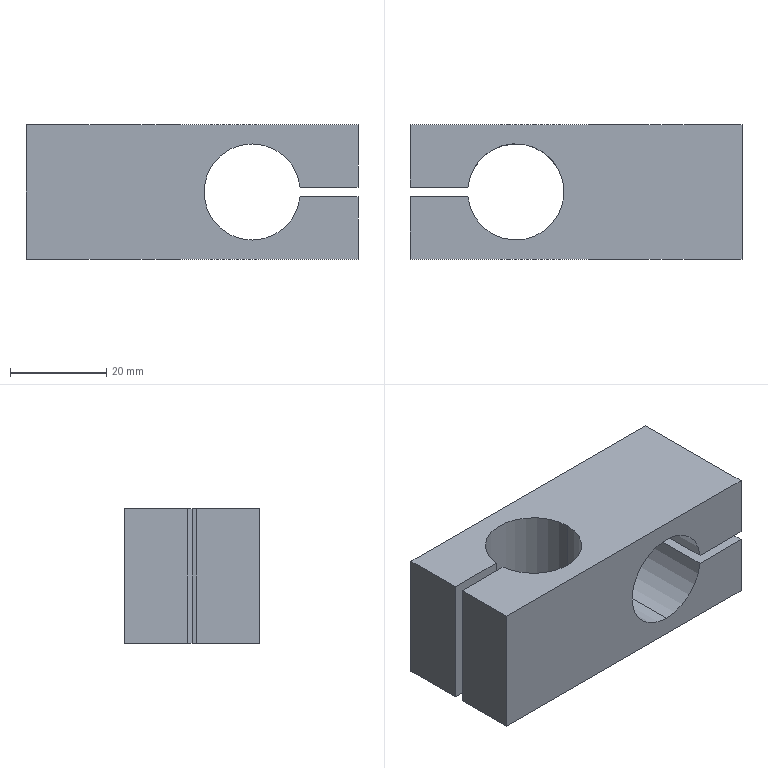Part | SolidWorks | features ICE 2, Extrusion 1 | 1 solid | 17 faces | box 69 x 28 x 28 mm | volume 35157 mm3 | plane 12 | cylinder 5 | commonest cylinder face diameters 20 x5
STEP:
#1=CARTESIAN_POINT('',(12.5,-14.,-10.));
#2=VERTEX_POINT('',#1);
#3=CARTESIAN_POINT('',(12.5,-14.,10.));
#4=VERTEX_POINT('',#3);
#5=CARTESIAN_POINT('',(12.5,-14.,0.));
#6=DIRECTION('',(0.,1.,0.));
#7=DIRECTION('',(0.,0.,1.));
#8=AXIS2_PLACEMENT_3D('',#5,#6,#7);
#9=CIRCLE('',#8,10.);
#10=EDGE_CURVE('',#2,#4,#9,.T.);
#11=ORIENTED_EDGE('',*,*,#10,.F.);
#12=CARTESIAN_POINT('',(12.5,14.,-10.));
#13=VERTEX_POINT('',#12);
#14=CARTESIAN_POINT('',(12.5,-14.,-10.));
#15=DIRECTION('',(0.,1.,0.));
#16=VECTOR('',#15,1000.);
#17=LINE('',#14,#16);
#18=EDGE_CURVE('',#2,#13,#17,.T.);
#19=ORIENTED_EDGE('',*,*,#18,.T.);
#20=CARTESIAN_POINT('',(12.5,14.,10.));
#21=VERTEX_POINT('',#20);
#22=CARTESIAN_POINT('',(12.5,14.,0.));
#23=DIRECTION('',(0.,1.,0.));
#24=DIRECTION('',(0.,0.,1.));
#25=AXIS2_PLACEMENT_3D('',#22,#23,#24);
#26=CIRCLE('',#25,10.);
#27=EDGE_CURVE('',#13,#21,#26,.T.);
#28=ORIENTED_EDGE('',*,*,#27,.T.);
#29=CARTESIAN_POINT('',(12.5,-14.,10.));
#30=DIRECTION('',(0.,1.,0.));
#31=VECTOR('',#30,1000.);
#32=LINE('',#29,#31);
#33=EDGE_CURVE('',#4,#21,#32,.T.);
#34=ORIENTED_EDGE('',*,*,#33,.F.);
#35=EDGE_LOOP('',(#11,#19,#28,#34));
#36=FACE_OUTER_BOUND('',#35,.T.);
#37=CARTESIAN_POINT('',(12.5,-14.,0.));
#38=DIRECTION('',(0.,1.,0.));
#39=DIRECTION('',(0.,0.,1.));
#40=AXIS2_PLACEMENT_3D('',#37,#38,#39);
#41=CYLINDRICAL_SURFACE('',#40,10.);
#42=ADVANCED_FACE('',(#36),#41,.F.);
#43=CARTESIAN_POINT('',(22.45,-14.,1.));
#44=VERTEX_POINT('',#43);
#45=CARTESIAN_POINT('',(12.5,-14.,0.));
#46=DIRECTION('',(0.,1.,0.));
#47=DIRECTION('',(0.,0.,1.));
#48=AXIS2_PLACEMENT_3D('',#45,#46,#47);
#49=CIRCLE('',#48,10.);
#50=EDGE_CURVE('',#4,#44,#49,.T.);
#51=ORIENTED_EDGE('',*,*,#50,.F.);
#52=ORIENTED_EDGE('',*,*,#33,.T.);
#53=CARTESIAN_POINT('',(22.45,14.,1.));
#54=VERTEX_POINT('',#53);
#55=CARTESIAN_POINT('',(12.5,14.,0.));
#56=DIRECTION('',(0.,1.,0.));
#57=DIRECTION('',(0.,0.,1.));
#58=AXIS2_PLACEMENT_3D('',#55,#56,#57);
#59=CIRCLE('',#58,10.);
#60=EDGE_CURVE('',#21,#54,#59,.T.);
#61=ORIENTED_EDGE('',*,*,#60,.T.);
#62=CARTESIAN_POINT('',(22.45,-14.,1.));
#63=DIRECTION('',(0.,1.,0.));
#64=VECTOR('',#63,1000.);
#65=LINE('',#62,#64);
#66=EDGE_CURVE('',#44,#54,#65,.T.);
#67=ORIENTED_EDGE('',*,*,#66,.F.);
#68=EDGE_LOOP('',(#51,#52,#61,#67));
#69=FACE_OUTER_BOUND('',#68,.T.);
#70=CARTESIAN_POINT('',(12.5,-14.,0.));
#71=DIRECTION('',(0.,1.,0.));
#72=DIRECTION('',(0.,0.,1.));
#73=AXIS2_PLACEMENT_3D('',#70,#71,#72);
#74=CYLINDRICAL_SURFACE('',#73,10.);
#75=ADVANCED_FACE('',(#69),#74,.F.);
#76=CARTESIAN_POINT('',(-2.5,0.,-14.));
#77=VERTEX_POINT('',#76);
#78=CARTESIAN_POINT('',(-22.45,1.,-14.));
#79=VERTEX_POINT('',#78);
#80=CARTESIAN_POINT('',(-12.5,0.,-14.));
#81=DIRECTION('',(0.,0.,1.));
#82=DIRECTION('',(1.,0.,0.));
#83=AXIS2_PLACEMENT_3D('',#80,#81,#82);
#84=CIRCLE('',#83,10.);
#85=EDGE_CURVE('',#77,#79,#84,.T.);
#86=ORIENTED_EDGE('',*,*,#85,.F.);
#87=CARTESIAN_POINT('',(-2.5,0.,14.));
#88=VERTEX_POINT('',#87);
#89=CARTESIAN_POINT('',(-2.5,0.,-14.));
#90=DIRECTION('',(0.,0.,1.));
#91=VECTOR('',#90,1000.);
#92=LINE('',#89,#91);
#93=EDGE_CURVE('',#77,#88,#92,.T.);
#94=ORIENTED_EDGE('',*,*,#93,.T.);
#95=CARTESIAN_POINT('',(-22.45,1.,14.));
#96=VERTEX_POINT('',#95);
#97=CARTESIAN_POINT('',(-12.5,0.,14.));
#98=DIRECTION('',(0.,0.,1.));
#99=DIRECTION('',(1.,0.,0.));
#100=AXIS2_PLACEMENT_3D('',#97,#98,#99);
#101=CIRCLE('',#100,10.);
#102=EDGE_CURVE('',#88,#96,#101,.T.);
#103=ORIENTED_EDGE('',*,*,#102,.T.);
#104=CARTESIAN_POINT('',(-22.45,1.,-14.));
#105=DIRECTION('',(0.,0.,1.));
#106=VECTOR('',#105,1000.);
#107=LINE('',#104,#106);
#108=EDGE_CURVE('',#79,#96,#107,.T.);
#109=ORIENTED_EDGE('',*,*,#108,.F.);
#110=EDGE_LOOP('',(#86,#94,#103,#109));
#111=FACE_OUTER_BOUND('',#110,.T.);
#112=CARTESIAN_POINT('',(-12.5,0.,-14.));
#113=DIRECTION('',(0.,0.,1.));
#114=DIRECTION('',(1.,0.,0.));
#115=AXIS2_PLACEMENT_3D('',#112,#113,#114);
#116=CYLINDRICAL_SURFACE('',#115,10.);
#117=ADVANCED_FACE('',(#111),#116,.F.);
#118=CARTESIAN_POINT('',(34.5,14.,-1.));
#119=VERTEX_POINT('',#118);
#120=CARTESIAN_POINT('',(34.5,14.,-14.));
#121=VERTEX_POINT('',#120);
#122=CARTESIAN_POINT('',(34.5,14.,14.));
#123=DIRECTION('',(0.,0.,-1.));
#124=VECTOR('',#123,1000.);
#125=LINE('',#122,#124);
#126=EDGE_CURVE('',#119,#121,#125,.T.);
#127=ORIENTED_EDGE('',*,*,#126,.F.);
#128=CARTESIAN_POINT('',(34.5,-14.,-1.));
#129=VERTEX_POINT('',#128);
#130=CARTESIAN_POINT('',(34.5,-14.,-1.));
#131=DIRECTION('',(0.,1.,0.));
#132=VECTOR('',#131,1000.);
#133=LINE('',#130,#132);
#134=EDGE_CURVE('',#129,#119,#133,.T.);
#135=ORIENTED_EDGE('',*,*,#134,.F.);
#136=CARTESIAN_POINT('',(34.5,-14.,-14.));
#137=VERTEX_POINT('',#136);
#138=CARTESIAN_POINT('',(34.5,-14.,14.));
#139=DIRECTION('',(0.,0.,-1.));
#140=VECTOR('',#139,1000.);
#141=LINE('',#138,#140);
#142=EDGE_CURVE('',#129,#137,#141,.T.);
#143=ORIENTED_EDGE('',*,*,#142,.T.);
#144=CARTESIAN_POINT('',(34.5,14.,-14.));
#145=DIRECTION('',(0.,1.,0.));
#146=VECTOR('',#145,1000.);
#147=LINE('',#144,#146);
#148=EDGE_CURVE('',#137,#121,#147,.T.);
#149=ORIENTED_EDGE('',*,*,#148,.T.);
#150=EDGE_LOOP('',(#127,#135,#143,#149));
#151=FACE_OUTER_BOUND('',#150,.T.);
#152=CARTESIAN_POINT('',(34.5,14.,14.));
#153=DIRECTION('',(-1.,0.,0.));
#154=DIRECTION('',(0.,0.,1.));
#155=AXIS2_PLACEMENT_3D('',#152,#153,#154);
#156=PLANE('',#155);
#157=ADVANCED_FACE('',(#151),#156,.F.);
#158=CARTESIAN_POINT('',(-34.5,14.,-14.));
#159=VERTEX_POINT('',#158);
#160=CARTESIAN_POINT('',(-34.5,1.,-14.));
#161=VERTEX_POINT('',#160);
#162=CARTESIAN_POINT('',(-34.5,14.,-14.));
#163=DIRECTION('',(0.,-1.,0.));
#164=VECTOR('',#163,1000.);
#165=LINE('',#162,#164);
#166=EDGE_CURVE('',#159,#161,#165,.T.);
#167=ORIENTED_EDGE('',*,*,#166,.T.);
#168=CARTESIAN_POINT('',(-34.5,1.,14.));
#169=VERTEX_POINT('',#168);
#170=CARTESIAN_POINT('',(-34.5,1.,-14.));
#171=DIRECTION('',(0.,0.,1.));
#172=VECTOR('',#171,1000.);
#173=LINE('',#170,#172);
#174=EDGE_CURVE('',#161,#169,#173,.T.);
#175=ORIENTED_EDGE('',*,*,#174,.T.);
#176=CARTESIAN_POINT('',(-34.5,14.,14.));
#177=VERTEX_POINT('',#176);
#178=CARTESIAN_POINT('',(-34.5,14.,14.));
#179=DIRECTION('',(0.,-1.,0.));
#180=VECTOR('',#179,1000.);
#181=LINE('',#178,#180);
#182=EDGE_CURVE('',#177,#169,#181,.T.);
#183=ORIENTED_EDGE('',*,*,#182,.F.);
#184=CARTESIAN_POINT('',(-34.5,14.,14.));
#185=DIRECTION('',(0.,0.,-1.));
#186=VECTOR('',#185,1000.);
#187=LINE('',#184,#186);
#188=EDGE_CURVE('',#177,#159,#187,.T.);
#189=ORIENTED_EDGE('',*,*,#188,.T.);
#190=EDGE_LOOP('',(#167,#175,#183,#189));
#191=FACE_OUTER_BOUND('',#190,.T.);
#192=CARTESIAN_POINT('',(-34.5,14.,14.));
#193=DIRECTION('',(1.,0.,0.));
#194=DIRECTION('',(0.,0.,-1.));
#195=AXIS2_PLACEMENT_3D('',#192,#193,#194);
#196=PLANE('',#195);
#197=ADVANCED_FACE('',(#191),#196,.F.);
#198=CARTESIAN_POINT('',(34.5,-14.,14.));
#199=VERTEX_POINT('',#198);
#200=CARTESIAN_POINT('',(34.5,-14.,1.));
#201=VERTEX_POINT('',#200);
#202=CARTESIAN_POINT('',(34.5,-14.,14.));
#203=DIRECTION('',(0.,0.,-1.));
#204=VECTOR('',#203,1000.);
#205=LINE('',#202,#204);
#206=EDGE_CURVE('',#199,#201,#205,.T.);
#207=ORIENTED_EDGE('',*,*,#206,.T.);
#208=CARTESIAN_POINT('',(34.5,14.,1.));
#209=VERTEX_POINT('',#208);
#210=CARTESIAN_POINT('',(34.5,-14.,1.));
#211=DIRECTION('',(0.,1.,0.));
#212=VECTOR('',#211,1000.);
#213=LINE('',#210,#212);
#214=EDGE_CURVE('',#201,#209,#213,.T.);
#215=ORIENTED_EDGE('',*,*,#214,.T.);
#216=CARTESIAN_POINT('',(34.5,14.,14.));
#217=VERTEX_POINT('',#216);
#218=CARTESIAN_POINT('',(34.5,14.,14.));
#219=DIRECTION('',(0.,0.,-1.));
#220=VECTOR('',#219,1000.);
#221=LINE('',#218,#220);
#222=EDGE_CURVE('',#217,#209,#221,.T.);
#223=ORIENTED_EDGE('',*,*,#222,.F.);
#224=CARTESIAN_POINT('',(34.5,14.,14.));
#225=DIRECTION('',(0.,1.,0.));
#226=VECTOR('',#225,1000.);
#227=LINE('',#224,#226);
#228=EDGE_CURVE('',#199,#217,#227,.T.);
#229=ORIENTED_EDGE('',*,*,#228,.F.);
#230=EDGE_LOOP('',(#207,#215,#223,#229));
#231=FACE_OUTER_BOUND('',#230,.T.);
#232=CARTESIAN_POINT('',(34.5,14.,14.));
#233=DIRECTION('',(-1.,0.,0.));
#234=DIRECTION('',(0.,0.,1.));
#235=AXIS2_PLACEMENT_3D('',#232,#233,#234);
#236=PLANE('',#235);
#237=ADVANCED_FACE('',(#231),#236,.F.);
#238=CARTESIAN_POINT('',(22.45,14.,-1.));
#239=VERTEX_POINT('',#238);
#240=CARTESIAN_POINT('',(12.5,14.,0.));
#241=DIRECTION('',(0.,1.,0.));
#242=DIRECTION('',(0.,0.,1.));
#243=AXIS2_PLACEMENT_3D('',#240,#241,#242);
#244=CIRCLE('',#243,10.);
#245=EDGE_CURVE('',#239,#13,#244,.T.);
#246=ORIENTED_EDGE('',*,*,#245,.F.);
#247=CARTESIAN_POINT('',(22.45,14.,-1.));
#248=DIRECTION('',(-1.,0.,0.));
#249=VECTOR('',#248,1000.);
#250=LINE('',#247,#249);
#251=EDGE_CURVE('',#119,#239,#250,.T.);
#252=ORIENTED_EDGE('',*,*,#251,.F.);
#253=ORIENTED_EDGE('',*,*,#126,.T.);
#254=CARTESIAN_POINT('',(-34.5,14.,-14.));
#255=DIRECTION('',(-1.,0.,0.));
#256=VECTOR('',#255,1000.);
#257=LINE('',#254,#256);
#258=EDGE_CURVE('',#121,#159,#257,.T.);
#259=ORIENTED_EDGE('',*,*,#258,.T.);
#260=ORIENTED_EDGE('',*,*,#188,.F.);
#261=CARTESIAN_POINT('',(-34.5,14.,14.));
#262=DIRECTION('',(-1.,0.,0.));
#263=VECTOR('',#262,1000.);
#264=LINE('',#261,#263);
#265=EDGE_CURVE('',#217,#177,#264,.T.);
#266=ORIENTED_EDGE('',*,*,#265,.F.);
#267=ORIENTED_EDGE('',*,*,#222,.T.);
#268=CARTESIAN_POINT('',(22.45,14.,1.));
#269=DIRECTION('',(1.,0.,0.));
#270=VECTOR('',#269,1000.);
#271=LINE('',#268,#270);
#272=EDGE_CURVE('',#54,#209,#271,.T.);
#273=ORIENTED_EDGE('',*,*,#272,.F.);
#274=ORIENTED_EDGE('',*,*,#60,.F.);
#275=ORIENTED_EDGE('',*,*,#27,.F.);
#276=EDGE_LOOP('',(#246,#252,#253,#259,#260,#266,#267,#273,#274,#275));
#277=FACE_OUTER_BOUND('',#276,.T.);
#278=CARTESIAN_POINT('',(-34.5,14.,14.));
#279=DIRECTION('',(0.,-1.,0.));
#280=DIRECTION('',(0.,0.,-1.));
#281=AXIS2_PLACEMENT_3D('',#278,#279,#280);
#282=PLANE('',#281);
#283=ADVANCED_FACE('',(#277),#282,.F.);
#284=CARTESIAN_POINT('',(-34.5,-1.,14.));
#285=VERTEX_POINT('',#284);
#286=CARTESIAN_POINT('',(-34.5,-14.,14.));
#287=VERTEX_POINT('',#286);
#288=CARTESIAN_POINT('',(-34.5,14.,14.));
#289=DIRECTION('',(0.,-1.,0.));
#290=VECTOR('',#289,1000.);
#291=LINE('',#288,#290);
#292=EDGE_CURVE('',#285,#287,#291,.T.);
#293=ORIENTED_EDGE('',*,*,#292,.F.);
#294=CARTESIAN_POINT('',(-34.5,-1.,-14.));
#295=VERTEX_POINT('',#294);
#296=CARTESIAN_POINT('',(-34.5,-1.,-14.));
#297=DIRECTION('',(0.,0.,1.));
#298=VECTOR('',#297,1000.);
#299=LINE('',#296,#298);
#300=EDGE_CURVE('',#295,#285,#299,.T.);
#301=ORIENTED_EDGE('',*,*,#300,.F.);
#302=CARTESIAN_POINT('',(-34.5,-14.,-14.));
#303=VERTEX_POINT('',#302);
#304=CARTESIAN_POINT('',(-34.5,14.,-14.));
#305=DIRECTION('',(0.,-1.,0.));
#306=VECTOR('',#305,1000.);
#307=LINE('',#304,#306);
#308=EDGE_CURVE('',#295,#303,#307,.T.);
#309=ORIENTED_EDGE('',*,*,#308,.T.);
#310=CARTESIAN_POINT('',(-34.5,-14.,14.));
#311=DIRECTION('',(0.,0.,-1.));
#312=VECTOR('',#311,1000.);
#313=LINE('',#310,#312);
#314=EDGE_CURVE('',#287,#303,#313,.T.);
#315=ORIENTED_EDGE('',*,*,#314,.F.);
#316=EDGE_LOOP('',(#293,#301,#309,#315));
#317=FACE_OUTER_BOUND('',#316,.T.);
#318=CARTESIAN_POINT('',(-34.5,14.,14.));
#319=DIRECTION('',(1.,0.,0.));
#320=DIRECTION('',(0.,0.,-1.));
#321=AXIS2_PLACEMENT_3D('',#318,#319,#320);
#322=PLANE('',#321);
#323=ADVANCED_FACE('',(#317),#322,.F.);
#324=ORIENTED_EDGE('',*,*,#142,.F.);
#325=CARTESIAN_POINT('',(22.45,-14.,-1.));
#326=VERTEX_POINT('',#325);
#327=CARTESIAN_POINT('',(22.45,-14.,-1.));
#328=DIRECTION('',(-1.,0.,0.));
#329=VECTOR('',#328,1000.);
#330=LINE('',#327,#329);
#331=EDGE_CURVE('',#129,#326,#330,.T.);
#332=ORIENTED_EDGE('',*,*,#331,.T.);
#333=CARTESIAN_POINT('',(12.5,-14.,0.));
#334=DIRECTION('',(0.,1.,0.));
#335=DIRECTION('',(0.,0.,1.));
#336=AXIS2_PLACEMENT_3D('',#333,#334,#335);
#337=CIRCLE('',#336,10.);
#338=EDGE_CURVE('',#326,#2,#337,.T.);
#339=ORIENTED_EDGE('',*,*,#338,.T.);
#340=ORIENTED_EDGE('',*,*,#10,.T.);
#341=ORIENTED_EDGE('',*,*,#50,.T.);
#342=CARTESIAN_POINT('',(22.45,-14.,1.));
#343=DIRECTION('',(1.,0.,0.));
#344=VECTOR('',#343,1000.);
#345=LINE('',#342,#344);
#346=EDGE_CURVE('',#44,#201,#345,.T.);
#347=ORIENTED_EDGE('',*,*,#346,.T.);
#348=ORIENTED_EDGE('',*,*,#206,.F.);
#349=CARTESIAN_POINT('',(-34.5,-14.,14.));
#350=DIRECTION('',(1.,0.,0.));
#351=VECTOR('',#350,1000.);
#352=LINE('',#349,#351);
#353=EDGE_CURVE('',#287,#199,#352,.T.);
#354=ORIENTED_EDGE('',*,*,#353,.F.);
#355=ORIENTED_EDGE('',*,*,#314,.T.);
#356=CARTESIAN_POINT('',(-34.5,-14.,-14.));
#357=DIRECTION('',(1.,0.,0.));
#358=VECTOR('',#357,1000.);
#359=LINE('',#356,#358);
#360=EDGE_CURVE('',#303,#137,#359,.T.);
#361=ORIENTED_EDGE('',*,*,#360,.T.);
#362=EDGE_LOOP('',(#324,#332,#339,#340,#341,#347,#348,#354,#355,#361));
#363=FACE_OUTER_BOUND('',#362,.T.);
#364=CARTESIAN_POINT('',(-34.5,-14.,14.));
#365=DIRECTION('',(0.,1.,0.));
#366=DIRECTION('',(0.,0.,1.));
#367=AXIS2_PLACEMENT_3D('',#364,#365,#366);
#368=PLANE('',#367);
#369=ADVANCED_FACE('',(#363),#368,.F.);
#370=CARTESIAN_POINT('',(-34.5,1.,14.));
#371=DIRECTION('',(-1.,0.,0.));
#372=VECTOR('',#371,1000.);
#373=LINE('',#370,#372);
#374=EDGE_CURVE('',#96,#169,#373,.T.);
#375=ORIENTED_EDGE('',*,*,#374,.F.);
#376=ORIENTED_EDGE('',*,*,#102,.F.);
#377=CARTESIAN_POINT('',(-22.45,-1.,14.));
#378=VERTEX_POINT('',#377);
#379=CARTESIAN_POINT('',(-12.5,0.,14.));
#380=DIRECTION('',(0.,0.,1.));
#381=DIRECTION('',(1.,0.,0.));
#382=AXIS2_PLACEMENT_3D('',#379,#380,#381);
#383=CIRCLE('',#382,10.);
#384=EDGE_CURVE('',#378,#88,#383,.T.);
#385=ORIENTED_EDGE('',*,*,#384,.F.);
#386=CARTESIAN_POINT('',(-34.5,-1.,14.));
#387=DIRECTION('',(1.,0.,0.));
#388=VECTOR('',#387,1000.);
#389=LINE('',#386,#388);
#390=EDGE_CURVE('',#285,#378,#389,.T.);
#391=ORIENTED_EDGE('',*,*,#390,.F.);
#392=ORIENTED_EDGE('',*,*,#292,.T.);
#393=ORIENTED_EDGE('',*,*,#353,.T.);
#394=ORIENTED_EDGE('',*,*,#228,.T.);
#395=ORIENTED_EDGE('',*,*,#265,.T.);
#396=ORIENTED_EDGE('',*,*,#182,.T.);
#397=EDGE_LOOP('',(#375,#376,#385,#391,#392,#393,#394,#395,#396));
#398=FACE_OUTER_BOUND('',#397,.T.);
#399=CARTESIAN_POINT('',(0.,0.,14.));
#400=DIRECTION('',(0.,0.,1.));
#401=DIRECTION('',(1.,0.,0.));
#402=AXIS2_PLACEMENT_3D('',#399,#400,#401);
#403=PLANE('',#402);
#404=ADVANCED_FACE('',(#398),#403,.T.);
#405=CARTESIAN_POINT('',(-22.45,-1.,-14.));
#406=VERTEX_POINT('',#405);
#407=CARTESIAN_POINT('',(-12.5,0.,-14.));
#408=DIRECTION('',(0.,0.,1.));
#409=DIRECTION('',(1.,0.,0.));
#410=AXIS2_PLACEMENT_3D('',#407,#408,#409);
#411=CIRCLE('',#410,10.);
#412=EDGE_CURVE('',#406,#77,#411,.T.);
#413=ORIENTED_EDGE('',*,*,#412,.T.);
#414=ORIENTED_EDGE('',*,*,#85,.T.);
#415=CARTESIAN_POINT('',(-34.5,1.,-14.));
#416=DIRECTION('',(-1.,0.,0.));
#417=VECTOR('',#416,1000.);
#418=LINE('',#415,#417);
#419=EDGE_CURVE('',#79,#161,#418,.T.);
#420=ORIENTED_EDGE('',*,*,#419,.T.);
#421=ORIENTED_EDGE('',*,*,#166,.F.);
#422=ORIENTED_EDGE('',*,*,#258,.F.);
#423=ORIENTED_EDGE('',*,*,#148,.F.);
#424=ORIENTED_EDGE('',*,*,#360,.F.);
#425=ORIENTED_EDGE('',*,*,#308,.F.);
#426=CARTESIAN_POINT('',(-34.5,-1.,-14.));
#427=DIRECTION('',(1.,0.,0.));
#428=VECTOR('',#427,1000.);
#429=LINE('',#426,#428);
#430=EDGE_CURVE('',#295,#406,#429,.T.);
#431=ORIENTED_EDGE('',*,*,#430,.T.);
#432=EDGE_LOOP('',(#413,#414,#420,#421,#422,#423,#424,#425,#431));
#433=FACE_OUTER_BOUND('',#432,.T.);
#434=CARTESIAN_POINT('',(0.,0.,-14.));
#435=DIRECTION('',(0.,0.,1.));
#436=DIRECTION('',(1.,0.,0.));
#437=AXIS2_PLACEMENT_3D('',#434,#435,#436);
#438=PLANE('',#437);
#439=ADVANCED_FACE('',(#433),#438,.F.);
#440=ORIENTED_EDGE('',*,*,#374,.T.);
#441=ORIENTED_EDGE('',*,*,#174,.F.);
#442=ORIENTED_EDGE('',*,*,#419,.F.);
#443=ORIENTED_EDGE('',*,*,#108,.T.);
#444=EDGE_LOOP('',(#440,#441,#442,#443));
#445=FACE_OUTER_BOUND('',#444,.T.);
#446=CARTESIAN_POINT('',(-34.5,1.,-14.));
#447=DIRECTION('',(0.,1.,0.));
#448=DIRECTION('',(0.,0.,1.));
#449=AXIS2_PLACEMENT_3D('',#446,#447,#448);
#450=PLANE('',#449);
#451=ADVANCED_FACE('',(#445),#450,.F.);
#452=ORIENTED_EDGE('',*,*,#93,.F.);
#453=ORIENTED_EDGE('',*,*,#412,.F.);
#454=CARTESIAN_POINT('',(-22.45,-1.,-14.));
#455=DIRECTION('',(0.,0.,1.));
#456=VECTOR('',#455,1000.);
#457=LINE('',#454,#456);
#458=EDGE_CURVE('',#406,#378,#457,.T.);
#459=ORIENTED_EDGE('',*,*,#458,.T.);
#460=ORIENTED_EDGE('',*,*,#384,.T.);
#461=EDGE_LOOP('',(#452,#453,#459,#460));
#462=FACE_OUTER_BOUND('',#461,.T.);
#463=CARTESIAN_POINT('',(-12.5,0.,-14.));
#464=DIRECTION('',(0.,0.,1.));
#465=DIRECTION('',(1.,0.,0.));
#466=AXIS2_PLACEMENT_3D('',#463,#464,#465);
#467=CYLINDRICAL_SURFACE('',#466,10.);
#468=ADVANCED_FACE('',(#462),#467,.F.);
#469=ORIENTED_EDGE('',*,*,#390,.T.);
#470=ORIENTED_EDGE('',*,*,#458,.F.);
#471=ORIENTED_EDGE('',*,*,#430,.F.);
#472=ORIENTED_EDGE('',*,*,#300,.T.);
#473=EDGE_LOOP('',(#469,#470,#471,#472));
#474=FACE_OUTER_BOUND('',#473,.T.);
#475=CARTESIAN_POINT('',(-34.5,-1.,-14.));
#476=DIRECTION('',(0.,-1.,0.));
#477=DIRECTION('',(0.,0.,-1.));
#478=AXIS2_PLACEMENT_3D('',#475,#476,#477);
#479=PLANE('',#478);
#480=ADVANCED_FACE('',(#474),#479,.F.);
#481=ORIENTED_EDGE('',*,*,#18,.F.);
#482=ORIENTED_EDGE('',*,*,#338,.F.);
#483=CARTESIAN_POINT('',(22.45,-14.,-1.));
#484=DIRECTION('',(0.,1.,0.));
#485=VECTOR('',#484,1000.);
#486=LINE('',#483,#485);
#487=EDGE_CURVE('',#326,#239,#486,.T.);
#488=ORIENTED_EDGE('',*,*,#487,.T.);
#489=ORIENTED_EDGE('',*,*,#245,.T.);
#490=EDGE_LOOP('',(#481,#482,#488,#489));
#491=FACE_OUTER_BOUND('',#490,.T.);
#492=CARTESIAN_POINT('',(12.5,-14.,0.));
#493=DIRECTION('',(0.,1.,0.));
#494=DIRECTION('',(0.,0.,1.));
#495=AXIS2_PLACEMENT_3D('',#492,#493,#494);
#496=CYLINDRICAL_SURFACE('',#495,10.);
#497=ADVANCED_FACE('',(#491),#496,.F.);
#498=ORIENTED_EDGE('',*,*,#251,.T.);
#499=ORIENTED_EDGE('',*,*,#487,.F.);
#500=ORIENTED_EDGE('',*,*,#331,.F.);
#501=ORIENTED_EDGE('',*,*,#134,.T.);
#502=EDGE_LOOP('',(#498,#499,#500,#501));
#503=FACE_OUTER_BOUND('',#502,.T.);
#504=CARTESIAN_POINT('',(22.45,-14.,-1.));
#505=DIRECTION('',(0.,0.,-1.));
#506=DIRECTION('',(-1.,0.,0.));
#507=AXIS2_PLACEMENT_3D('',#504,#505,#506);
#508=PLANE('',#507);
#509=ADVANCED_FACE('',(#503),#508,.F.);
#510=ORIENTED_EDGE('',*,*,#272,.T.);
#511=ORIENTED_EDGE('',*,*,#214,.F.);
#512=ORIENTED_EDGE('',*,*,#346,.F.);
#513=ORIENTED_EDGE('',*,*,#66,.T.);
#514=EDGE_LOOP('',(#510,#511,#512,#513));
#515=FACE_OUTER_BOUND('',#514,.T.);
#516=CARTESIAN_POINT('',(22.45,-14.,1.));
#517=DIRECTION('',(0.,0.,1.));
#518=DIRECTION('',(1.,0.,0.));
#519=AXIS2_PLACEMENT_3D('',#516,#517,#518);
#520=PLANE('',#519);
#521=ADVANCED_FACE('',(#515),#520,.F.);
#522=CLOSED_SHELL('',(#42,#75,#117,#157,#197,#237,#283,#323,#369,#404,#439,#451,#468,#480,#497,#509,#521));
#523=MANIFOLD_SOLID_BREP('',#522);
#524=CARTESIAN_POINT('',(0.,0.,0.));
#525=DIRECTION('',(0.,0.,1.));
#526=DIRECTION('',(1.,0.,0.));
#527=AXIS2_PLACEMENT_3D('',#524,#525,#526);
#528=(LENGTH_UNIT()NAMED_UNIT(*)SI_UNIT(.MILLI.,.METRE.));
#529=UNCERTAINTY_MEASURE_WITH_UNIT(LENGTH_MEASURE(0.00001),#528,'','');
#530=(NAMED_UNIT(*)PLANE_ANGLE_UNIT()SI_UNIT($,.RADIAN.));
#531=(NAMED_UNIT(*)SI_UNIT($,.STERADIAN.)SOLID_ANGLE_UNIT());
#532=(GEOMETRIC_REPRESENTATION_CONTEXT(3)GLOBAL_UNCERTAINTY_ASSIGNED_CONTEXT((#529))GLOBAL_UNIT_ASSIGNED_CONTEXT((#528,#530,#531))REPRESENTATION_CONTEXT('',''));
#533=ADVANCED_BREP_SHAPE_REPRESENTATION('',(#523,#527),#532);